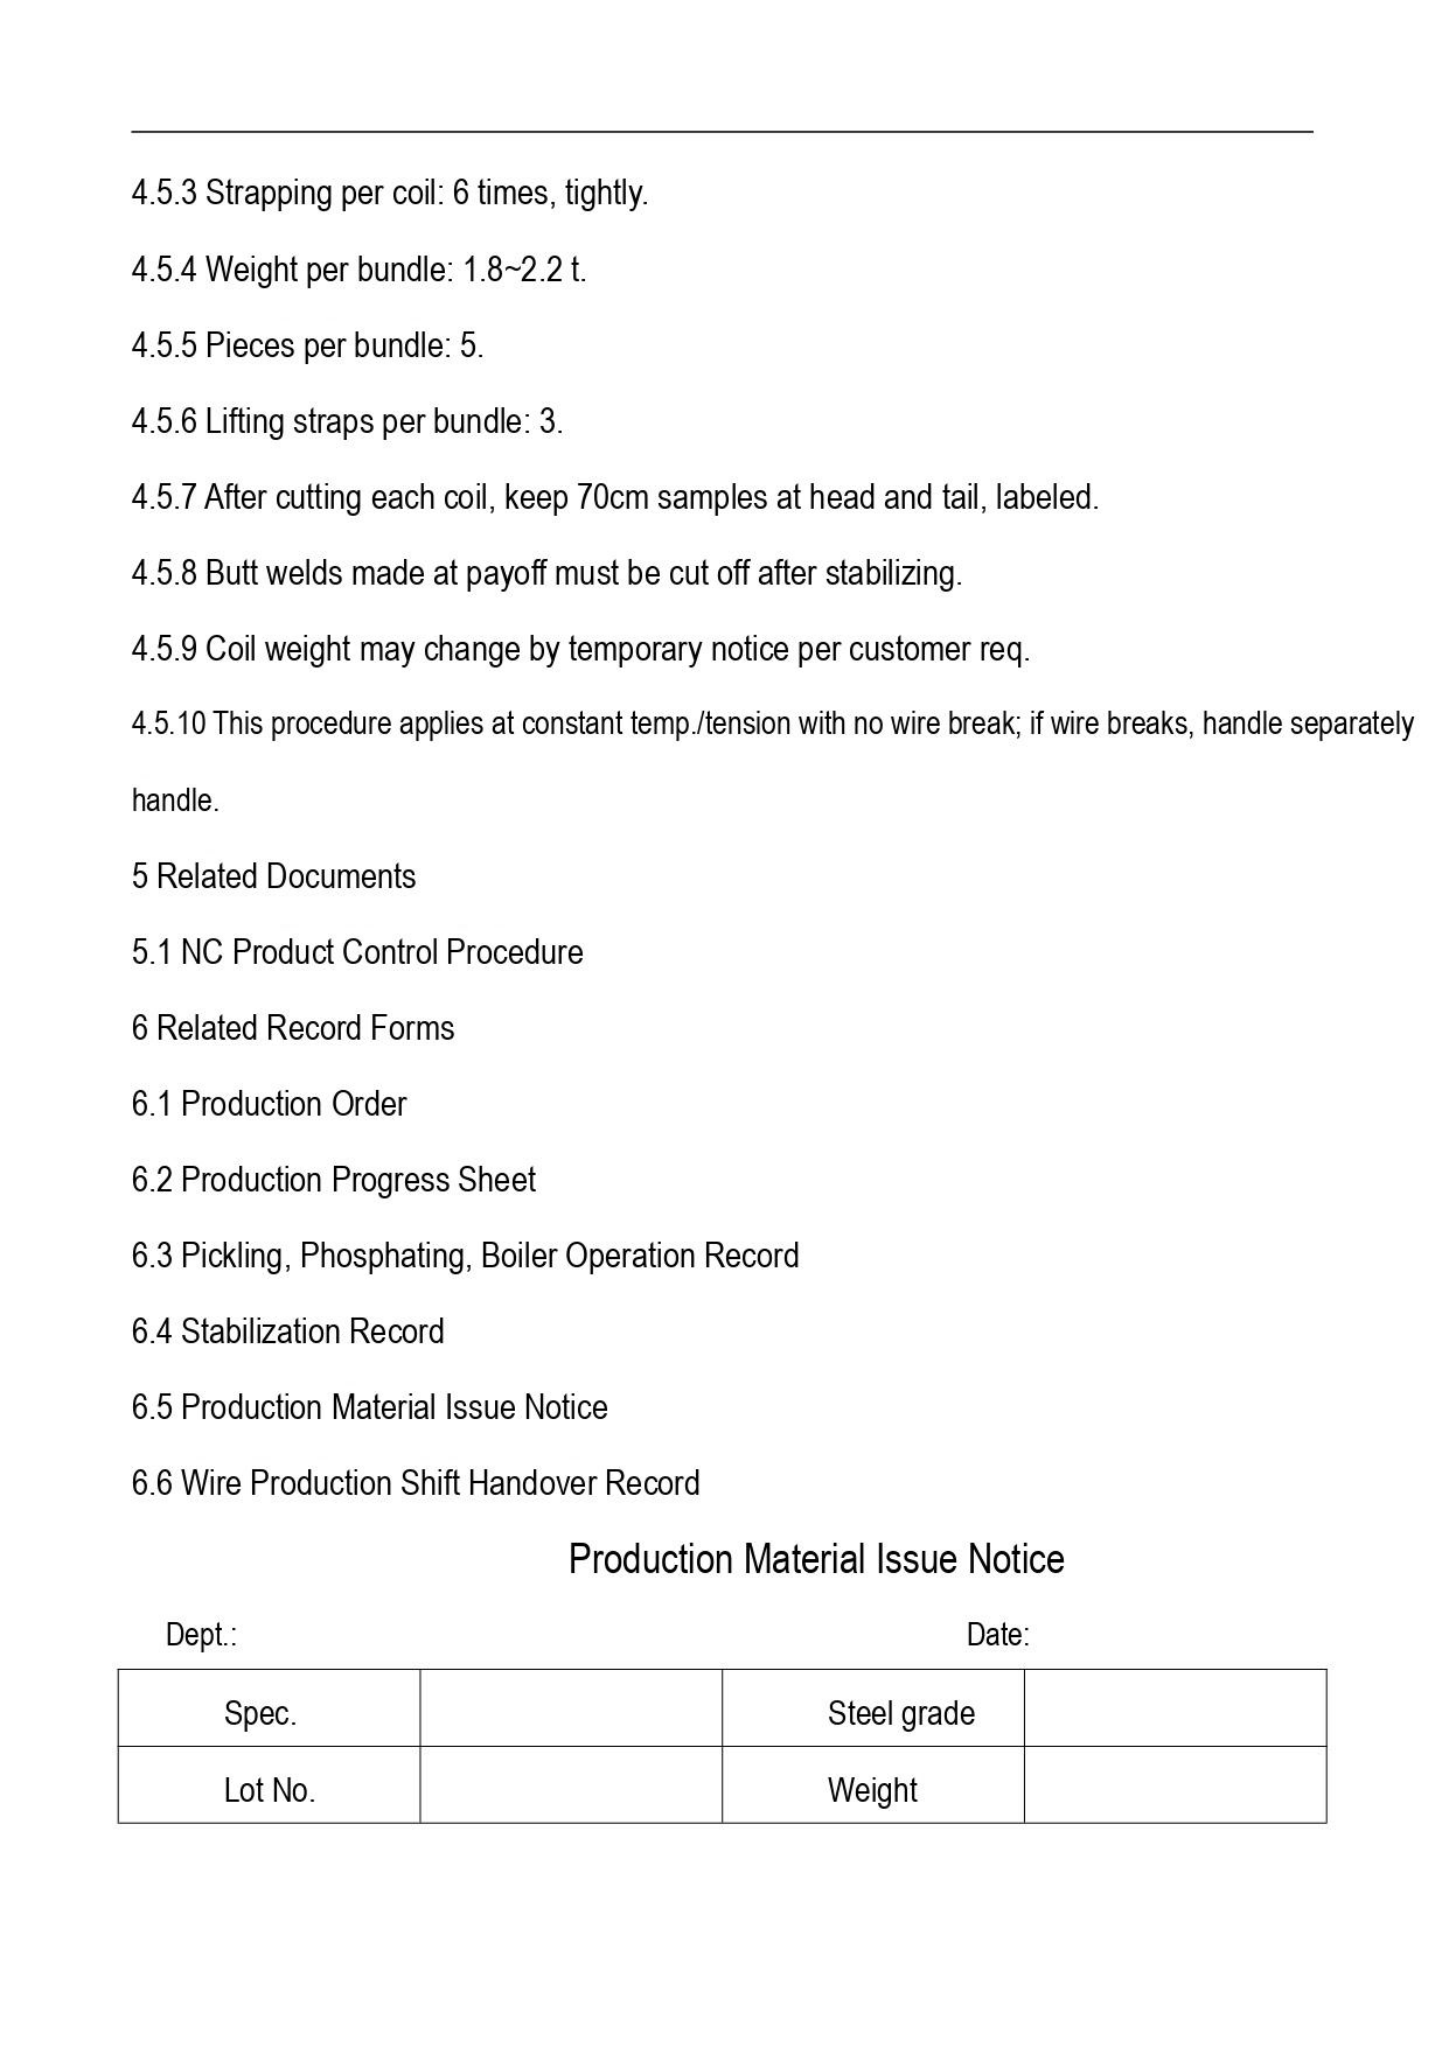4.5.3 Strapping per coil: 6 times, tightly.

4.5.4 Weight per bundle: 1.8~2.2 t.

4.5.5 Pieces per bundle: 5.

4.5.6 Lifting straps per bundle: 3.

4.5.7 After cutting each coil, keep 70cm samples at head and tail, labeled.

4.5.8 Butt welds made at payoff must be cut off after stabilizing.

4.5.9 Coil weight may change by temporary notice per customer req.

4.5.10 This procedure applies at constant temp./tension with no wire break; if wire breaks, handle separately handle.

5 Related Documents

5.1 NC Product Control Procedure

6 Related Record Forms

6.1 Production Order

6.2 Production Progress Sheet

6.3 Pickling, Phosphating, Boiler Operation Record

6.4 Stabilization Record

6.5 Production Material Issue Notice

6.6 Wire Production Shift Handover Record

Production Material Issue Notice

Dept.: Date:

| Spec. | | Steel grade | |
|---|---|---|---|
| Lot No. | | Weight | |
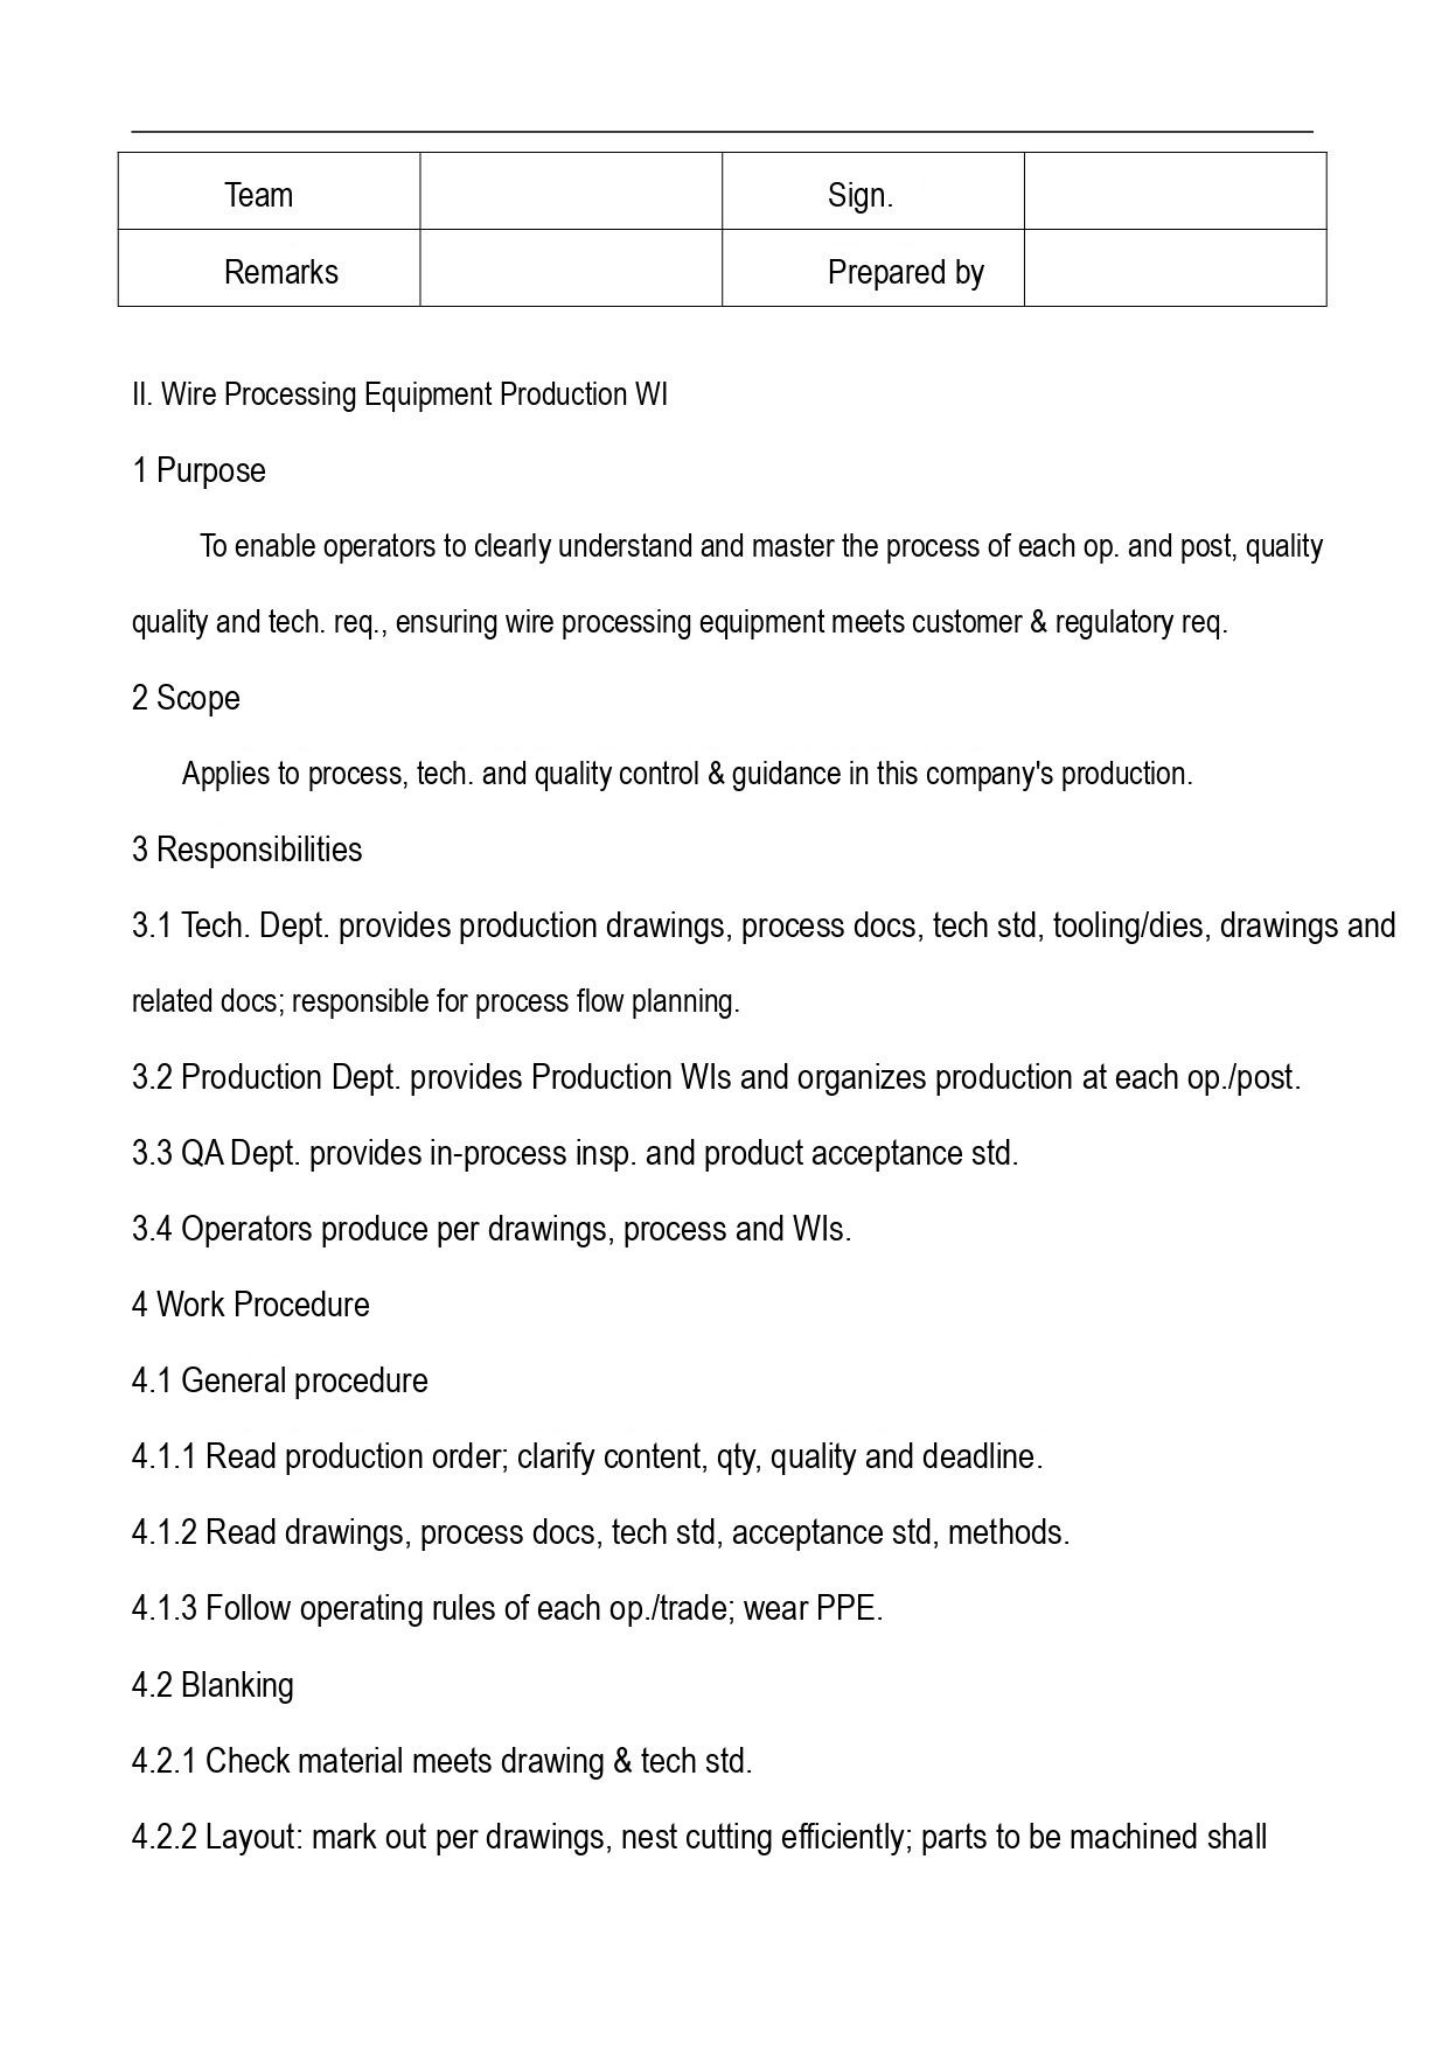| Team |  | Sign. |  |
|---|---|---|---|
| Remarks |  | Prepared by |  |

II. Wire Processing Equipment Production WI

1 Purpose

To enable operators to clearly understand and master the process of each op. and post, quality quality and tech. req., ensuring wire processing equipment meets customer & regulatory req.

2 Scope

Applies to process, tech. and quality control & guidance in this company's production.

3 Responsibilities

3.1 Tech. Dept. provides production drawings, process docs, tech std, tooling/dies, drawings and related docs; responsible for process flow planning.

3.2 Production Dept. provides Production WIs and organizes production at each op./post.

3.3 QA Dept. provides in-process insp. and product acceptance std.

3.4 Operators produce per drawings, process and WIs.

4 Work Procedure

4.1 General procedure

4.1.1 Read production order; clarify content, qty, quality and deadline.

4.1.2 Read drawings, process docs, tech std, acceptance std, methods.

4.1.3 Follow operating rules of each op./trade; wear PPE.

4.2 Blanking

4.2.1 Check material meets drawing & tech std.

4.2.2 Layout: mark out per drawings, nest cutting efficiently; parts to be machined shall
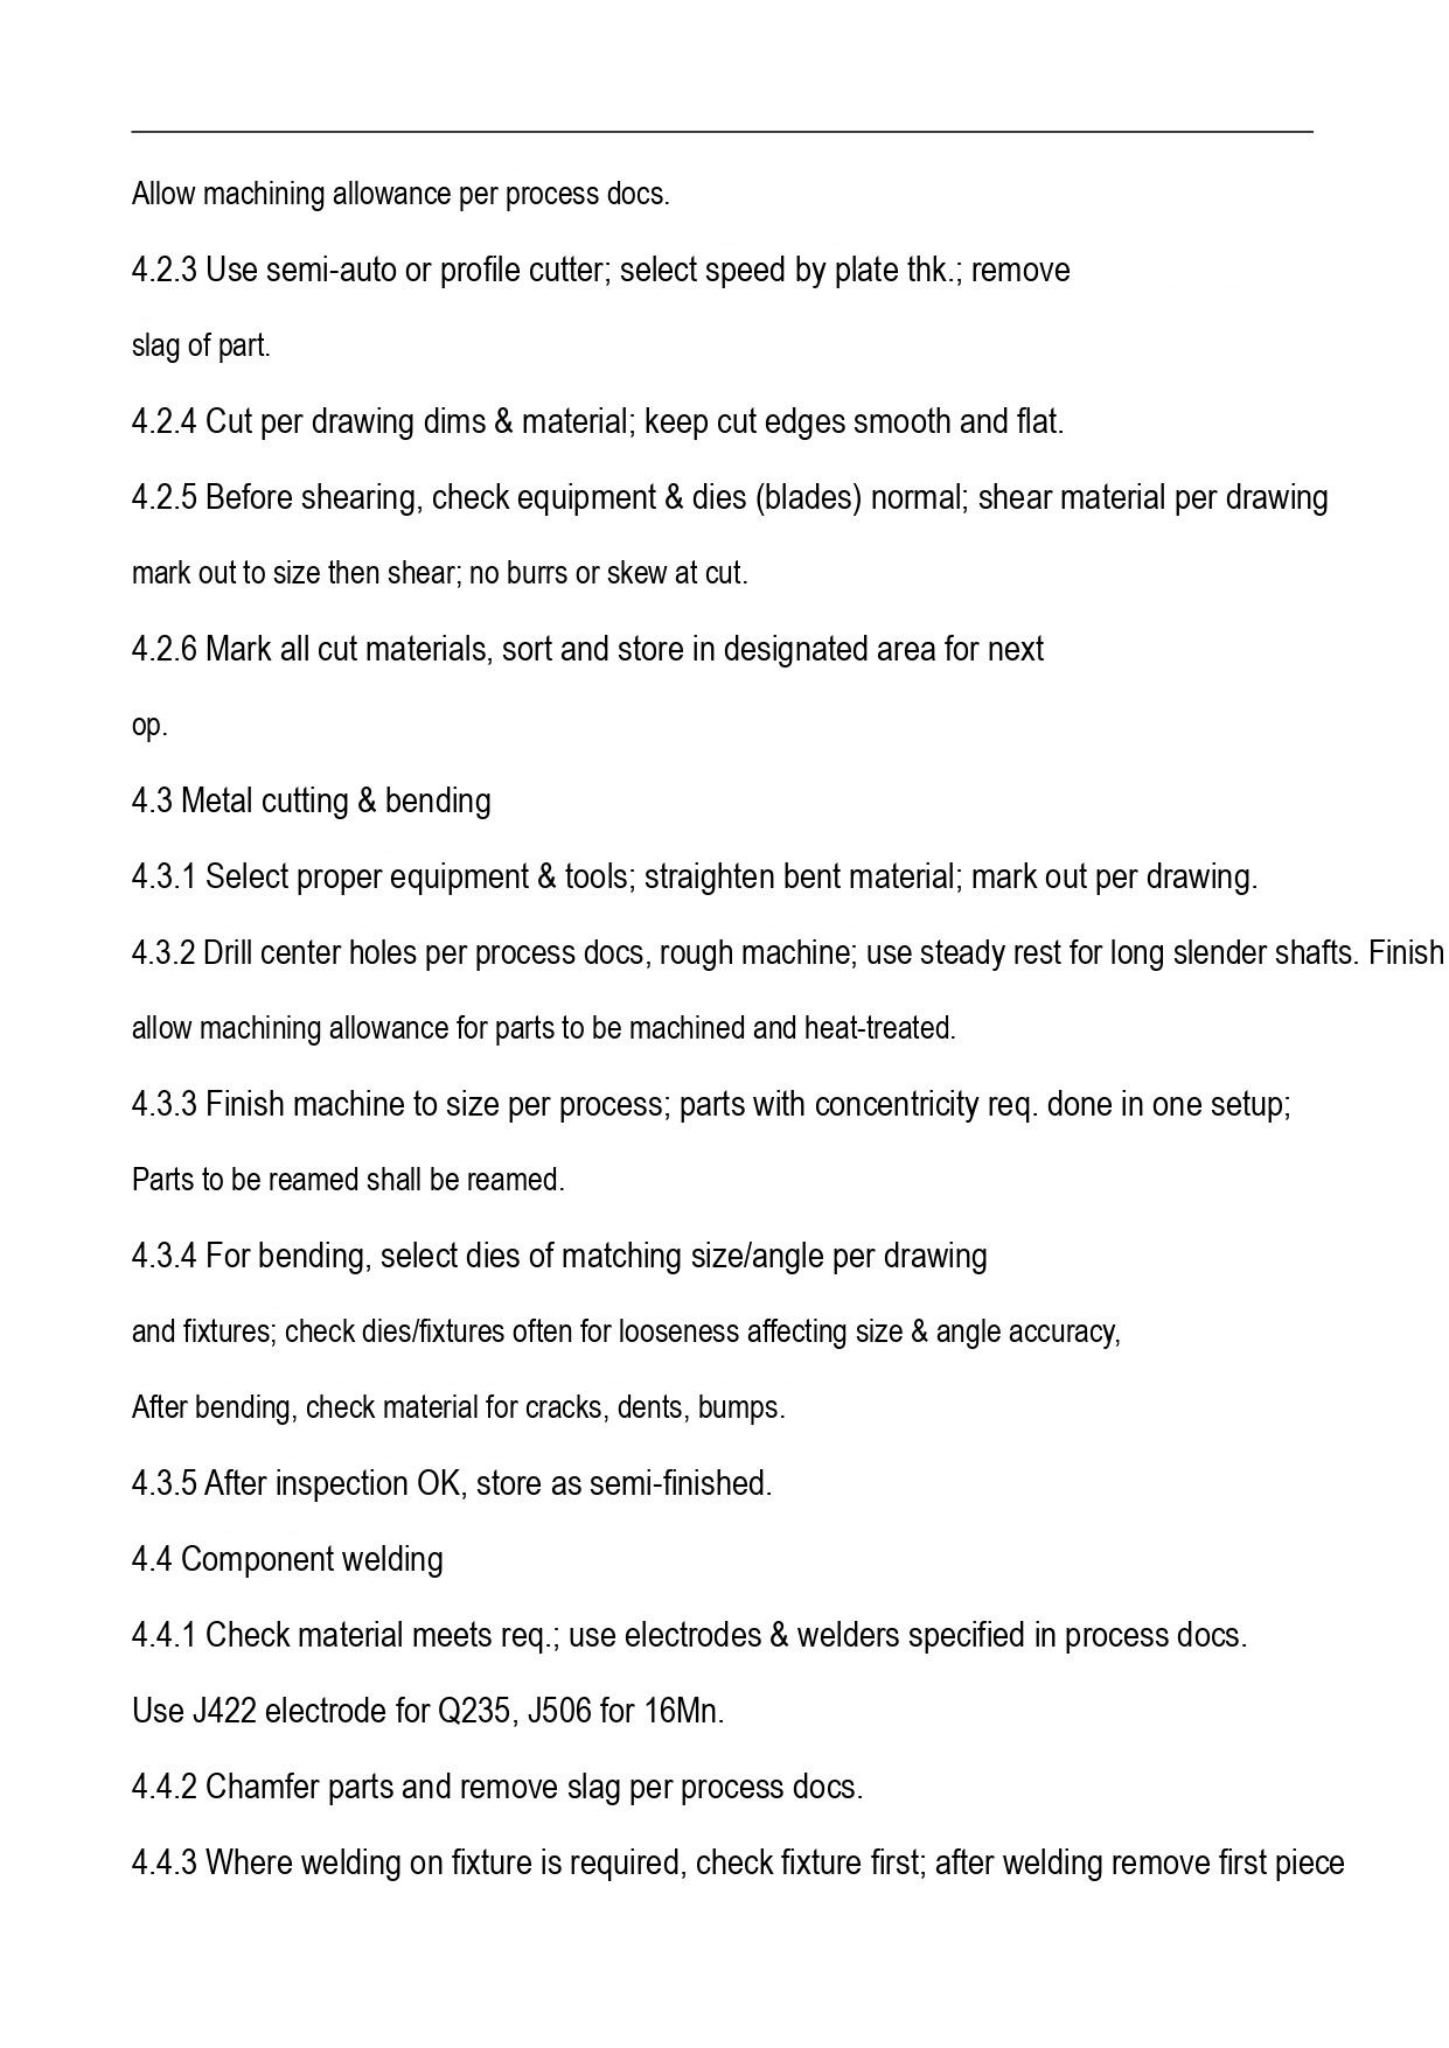Allow machining allowance per process docs.

4.2.3 Use semi-auto or profile cutter; select speed by plate thk.; remove

slag of part.

4.2.4 Cut per drawing dims & material; keep cut edges smooth and flat.

4.2.5 Before shearing, check equipment & dies (blades) normal; shear material per drawing

mark out to size then shear; no burrs or skew at cut.

4.2.6 Mark all cut materials, sort and store in designated area for next

op.

4.3 Metal cutting & bending

4.3.1 Select proper equipment & tools; straighten bent material; mark out per drawing.

4.3.2 Drill center holes per process docs, rough machine; use steady rest for long slender shafts. Finish

allow machining allowance for parts to be machined and heat-treated.

4.3.3 Finish machine to size per process; parts with concentricity req. done in one setup;

Parts to be reamed shall be reamed.

4.3.4 For bending, select dies of matching size/angle per drawing

and fixtures; check dies/fixtures often for looseness affecting size & angle accuracy,

After bending, check material for cracks, dents, bumps.

4.3.5 After inspection OK, store as semi-finished.

4.4 Component welding

4.4.1 Check material meets req.; use electrodes & welders specified in process docs.

Use J422 electrode for Q235, J506 for 16Mn.

4.4.2 Chamfer parts and remove slag per process docs.

4.4.3 Where welding on fixture is required, check fixture first; after welding remove first piece
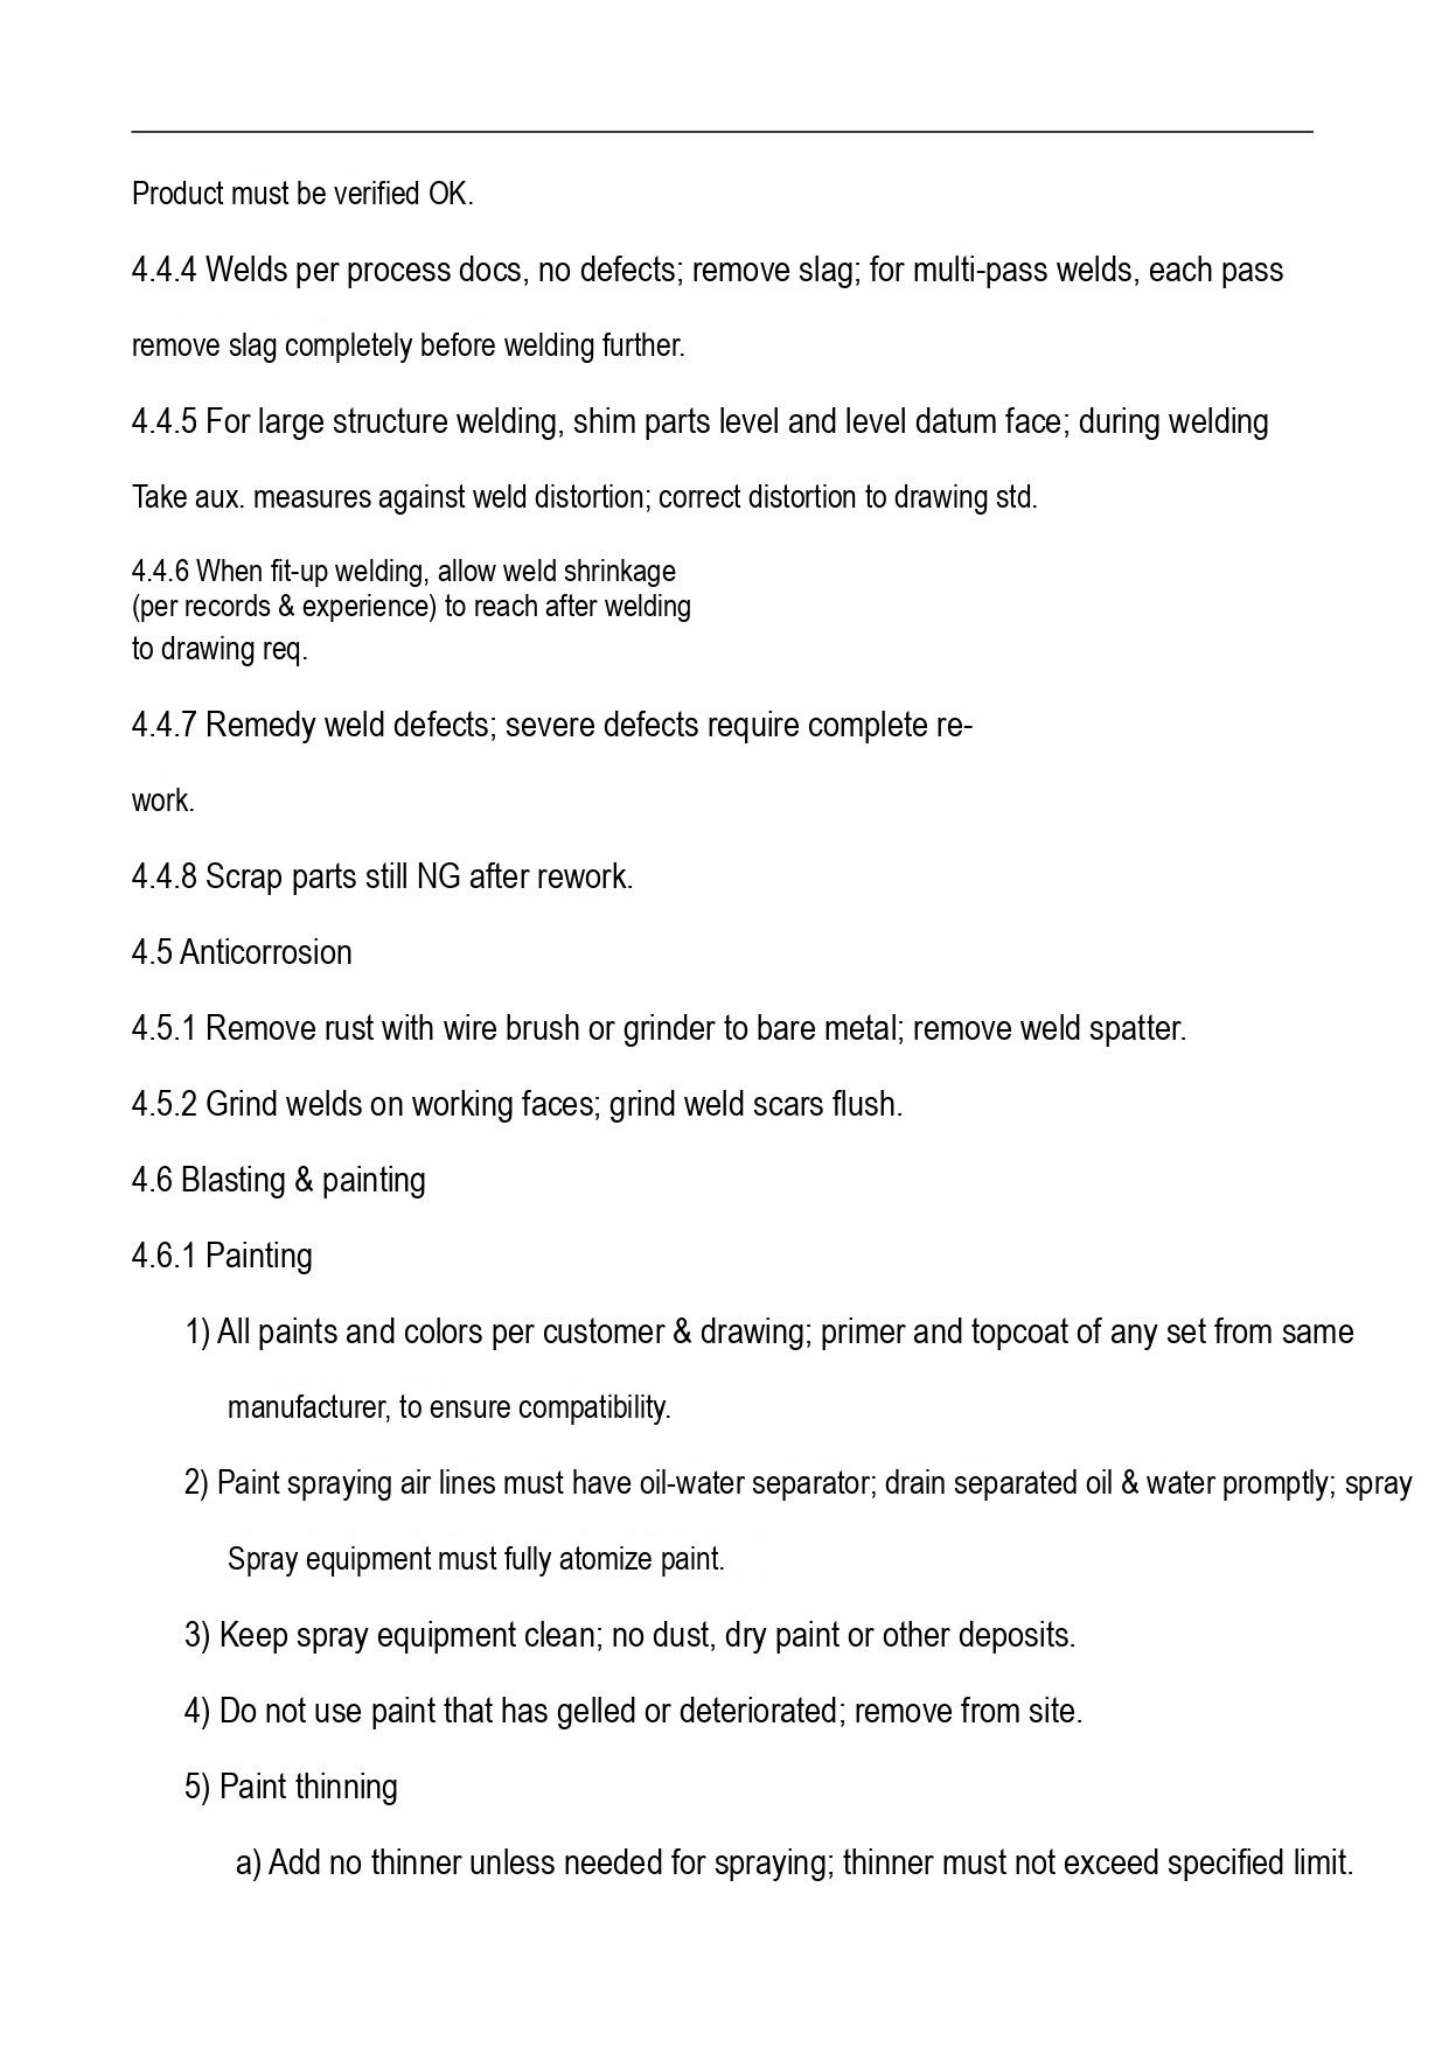Product must be verified OK.

4.4.4 Welds per process docs, no defects; remove slag; for multi-pass welds, each pass

remove slag completely before welding further.

4.4.5 For large structure welding, shim parts level and level datum face; during welding

Take aux. measures against weld distortion; correct distortion to drawing std.

4.4.6 When fit-up welding, allow weld shrinkage
(per records & experience) to reach after welding
to drawing req.

4.4.7 Remedy weld defects; severe defects require complete re-

work.

4.4.8 Scrap parts still NG after rework.

4.5 Anticorrosion

4.5.1 Remove rust with wire brush or grinder to bare metal; remove weld spatter.

4.5.2 Grind welds on working faces; grind weld scars flush.

4.6 Blasting & painting

4.6.1 Painting

1) All paints and colors per customer & drawing; primer and topcoat of any set from same

manufacturer, to ensure compatibility.

2) Paint spraying air lines must have oil-water separator; drain separated oil & water promptly; spray

Spray equipment must fully atomize paint.

3) Keep spray equipment clean; no dust, dry paint or other deposits.

4) Do not use paint that has gelled or deteriorated; remove from site.

5) Paint thinning

a) Add no thinner unless needed for spraying; thinner must not exceed specified limit.
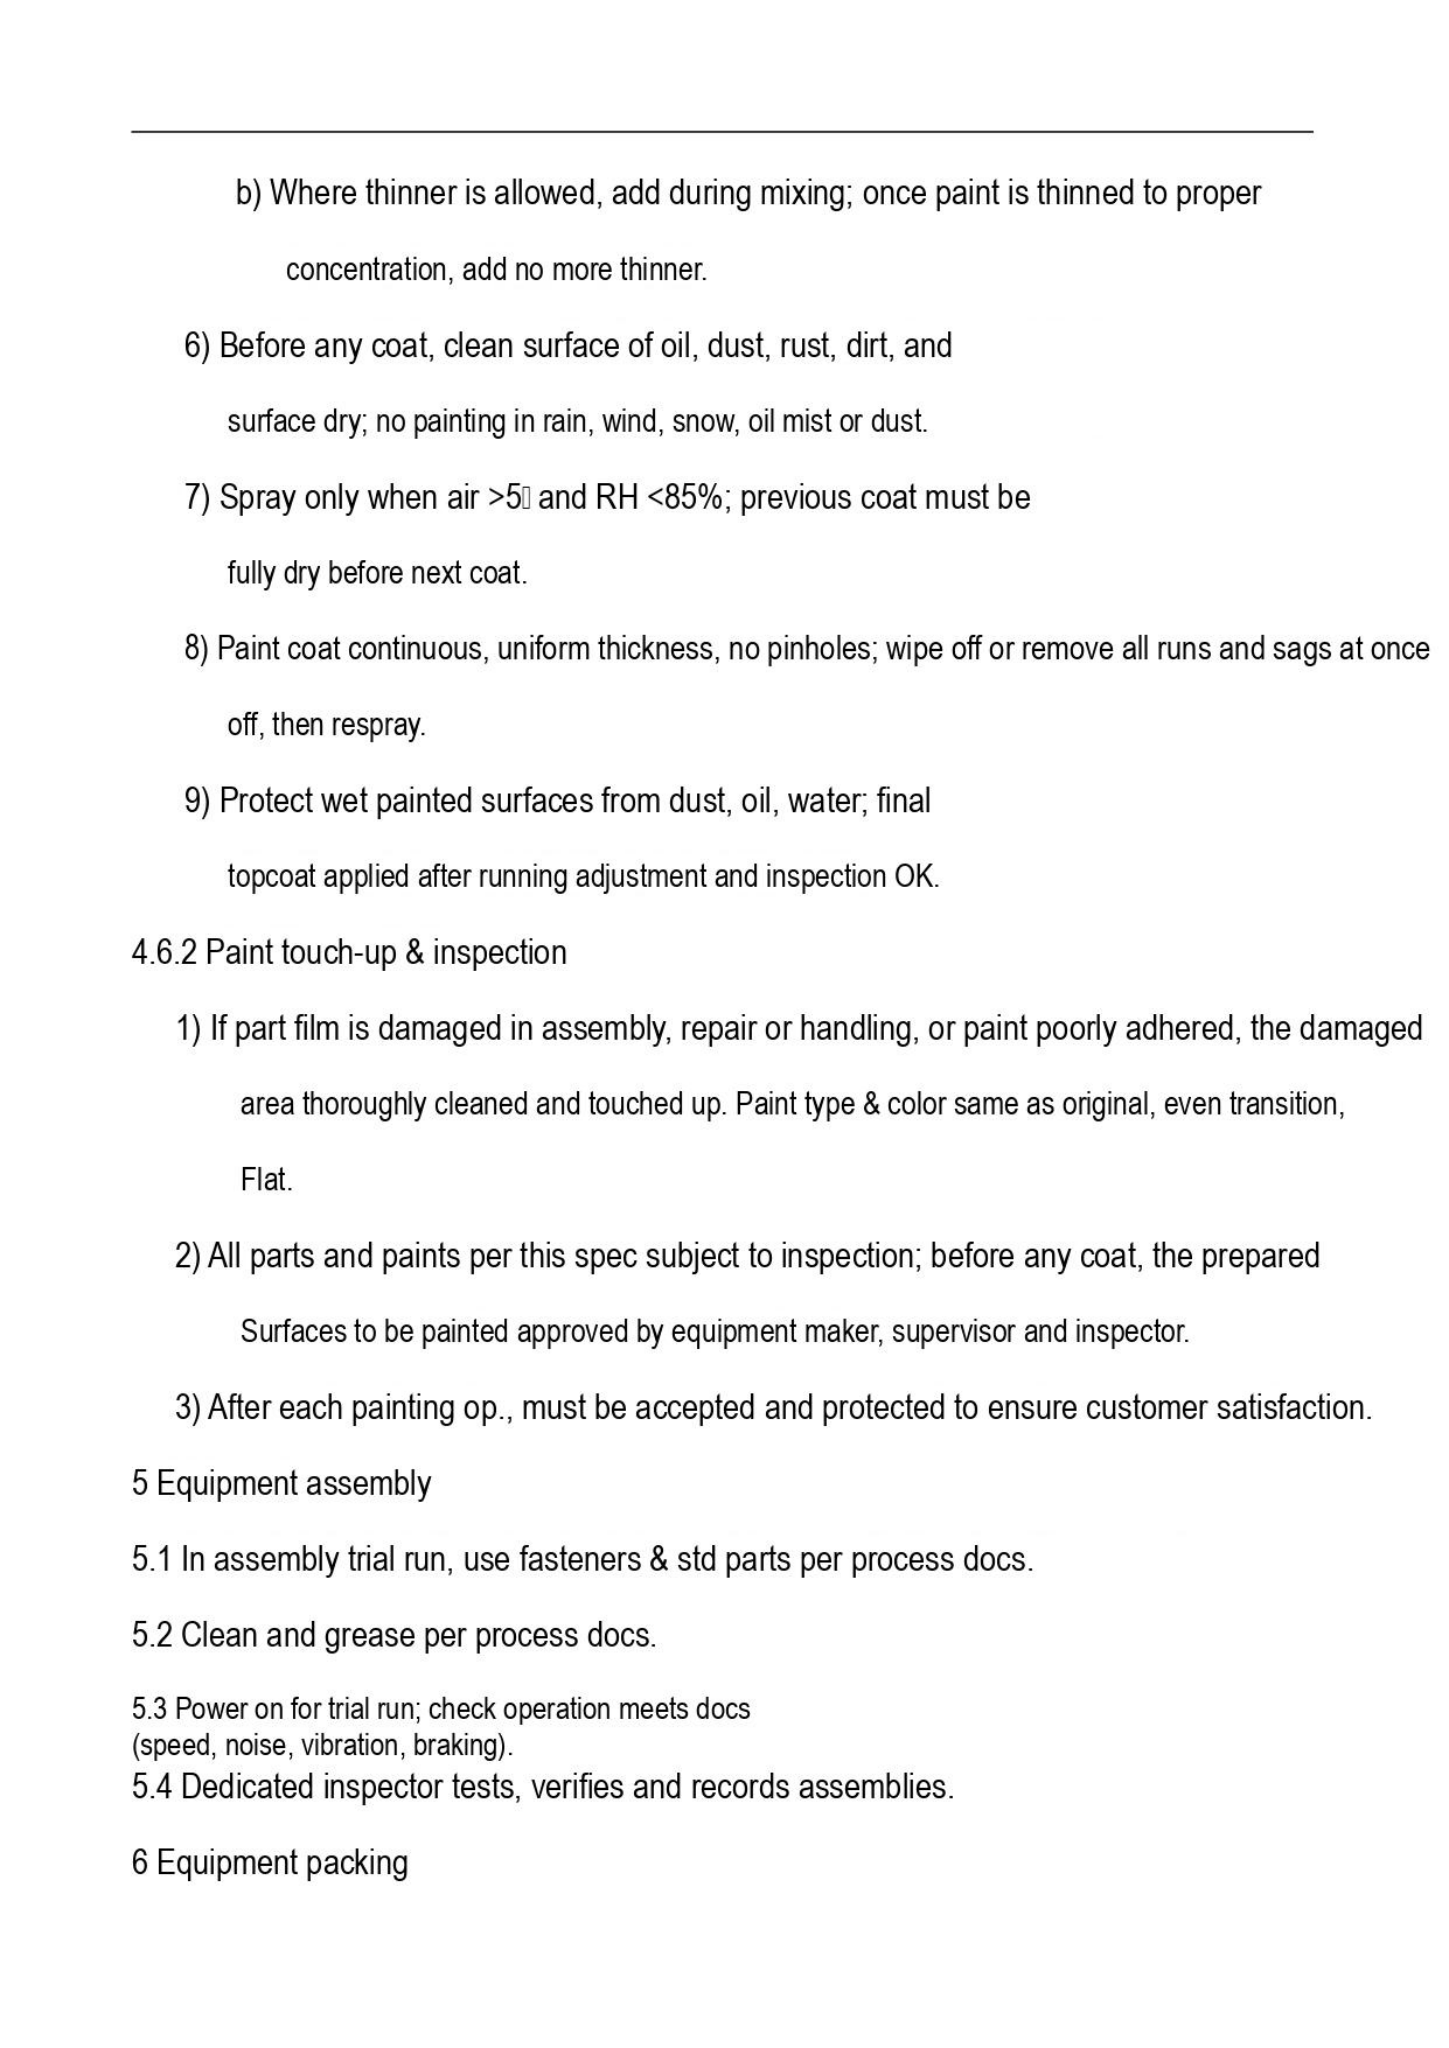b) Where thinner is allowed, add during mixing; once paint is thinned to proper

concentration, add no more thinner.

6) Before any coat, clean surface of oil, dust, rust, dirt, and

surface dry; no painting in rain, wind, snow, oil mist or dust.

7) Spray only when air >5 and RH <85%; previous coat must be

fully dry before next coat.

8) Paint coat continuous, uniform thickness, no pinholes; wipe off or remove all runs and sags at once

off, then respray.

9) Protect wet painted surfaces from dust, oil, water; final

topcoat applied after running adjustment and inspection OK.

4.6.2 Paint touch-up & inspection

1) If part film is damaged in assembly, repair or handling, or paint poorly adhered, the damaged

area thoroughly cleaned and touched up. Paint type & color same as original, even transition,

Flat.

2) All parts and paints per this spec subject to inspection; before any coat, the prepared

Surfaces to be painted approved by equipment maker, supervisor and inspector.

3) After each painting op., must be accepted and protected to ensure customer satisfaction.

5 Equipment assembly

5.1 In assembly trial run, use fasteners & std parts per process docs.

5.2 Clean and grease per process docs.

5.3 Power on for trial run; check operation meets docs
(speed, noise, vibration, braking).

5.4 Dedicated inspector tests, verifies and records assemblies.

6 Equipment packing
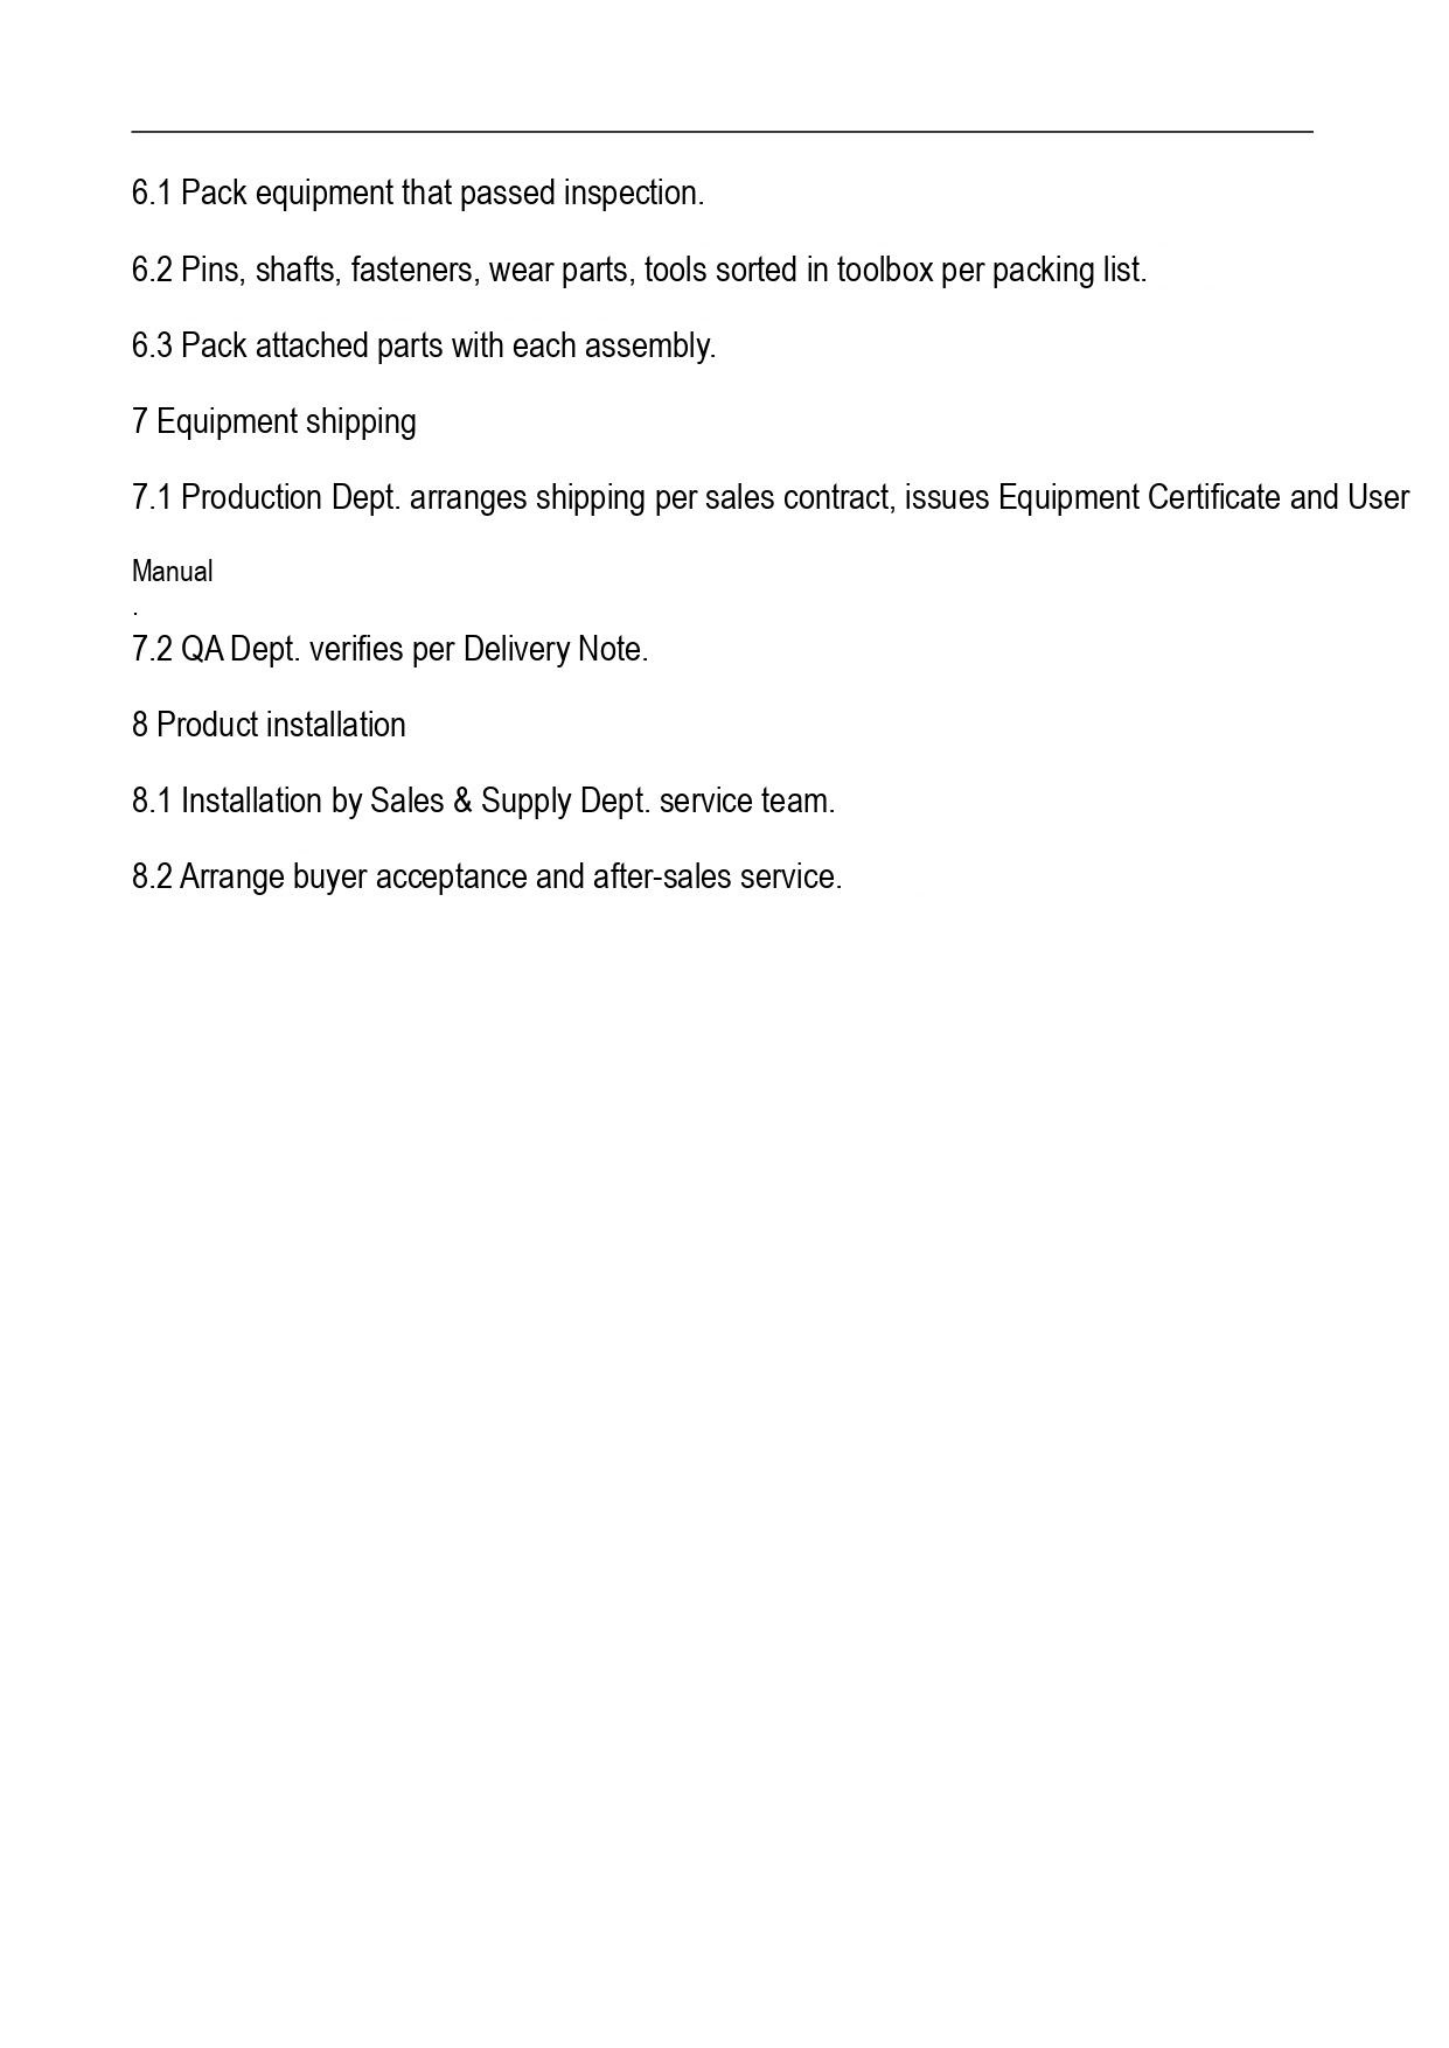6.1 Pack equipment that passed inspection.

6.2 Pins, shafts, fasteners, wear parts, tools sorted in toolbox per packing list.

6.3 Pack attached parts with each assembly.

7 Equipment shipping

7.1 Production Dept. arranges shipping per sales contract, issues Equipment Certificate and User Manual
.

7.2 QA Dept. verifies per Delivery Note.

8 Product installation

8.1 Installation by Sales & Supply Dept. service team.

8.2 Arrange buyer acceptance and after-sales service.